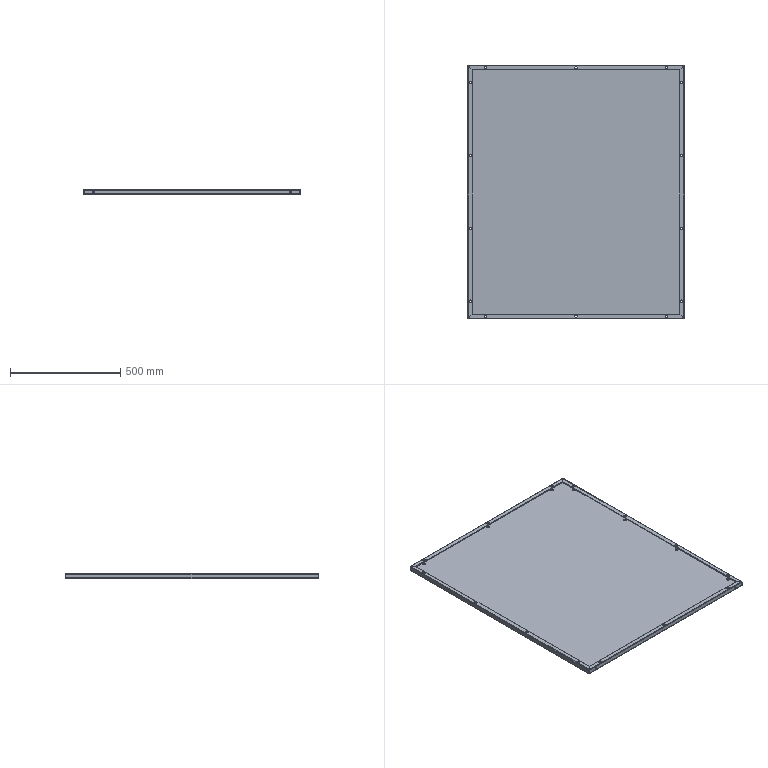Part | STEP file | 750038381 | 1 solid | 137 faces | box 981 x 1150 x 23 mm | volume 1927525 mm3 | cylinder 77 | plane 46 | spline 14 | commonest cylinder face diameters 12 x56 3 x8 6 x8 9 x4 2 x1